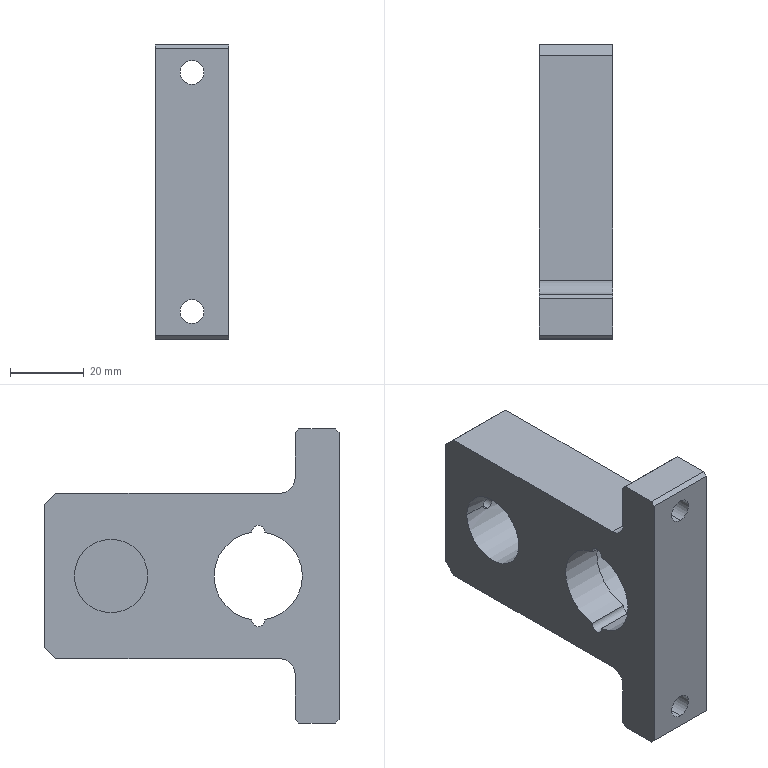Part | STEP file | Small support plate_sand-blasted, oxidised | 1 solid | 52 faces | box 20 x 80 x 80 mm | volume 64176 mm3 | cylinder 26 | plane 18 | cone 8 | commonest cylinder face diameters 3.3 x10 6.5 x4 3.5 x3 24 x3 8 x2 20 x2